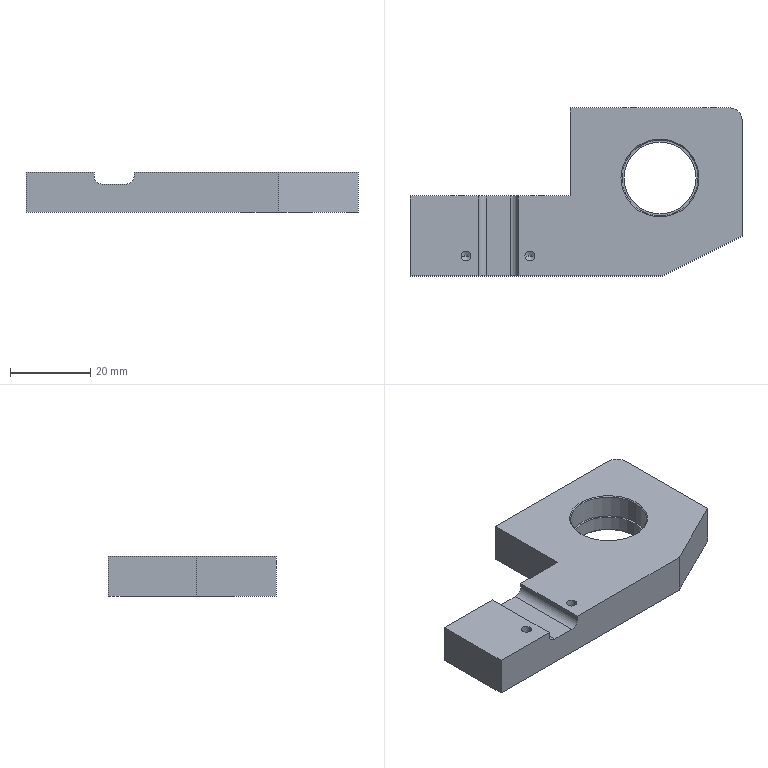Part | NX | features BREP 1 | 1 solid | 49 faces | box 83 x 42 x 10 mm | volume 21285 mm3 | cylinder 19 | cone 16 | plane 14 | commonest cylinder face diameters 3.3 x8 2.5 x4 4 x2 18 x2 19 x2 6 x1
STEP:
#1=CARTESIAN_POINT('',(15.,10.909,0.));
#2=VERTEX_POINT('',#1);
#3=CARTESIAN_POINT('',(15.,11.9,-1.65));
#4=VERTEX_POINT('',#3);
#5=CARTESIAN_POINT('',(15.,11.9,-1.65));
#6=DIRECTION('',(0.,0.515,-0.8572));
#7=VECTOR('',#6,1000.);
#8=LINE('',#5,#7);
#9=EDGE_CURVE('',#2,#4,#8,.T.);
#10=ORIENTED_EDGE('',*,*,#9,.F.);
#11=CARTESIAN_POINT('',(15.,11.9,1.65));
#12=VERTEX_POINT('',#11);
#13=CARTESIAN_POINT('',(15.,11.9,1.65));
#14=DIRECTION('',(0.,0.515,0.8572));
#15=VECTOR('',#14,1000.);
#16=LINE('',#13,#15);
#17=EDGE_CURVE('',#2,#12,#16,.T.);
#18=ORIENTED_EDGE('',*,*,#17,.T.);
#19=CARTESIAN_POINT('',(16.543,11.9,0.5854));
#20=VERTEX_POINT('',#19);
#21=CARTESIAN_POINT('',(15.,11.9,0.));
#22=DIRECTION('',(0.,1.,0.));
#23=DIRECTION('',(0.,0.,1.));
#24=AXIS2_PLACEMENT_3D('',#21,#22,#23);
#25=CIRCLE('',#24,1.65);
#26=EDGE_CURVE('',#12,#20,#25,.T.);
#27=ORIENTED_EDGE('',*,*,#26,.T.);
#28=CARTESIAN_POINT('',(16.543,11.9,-0.5854));
#29=VERTEX_POINT('',#28);
#30=CARTESIAN_POINT('',(16.543,11.9,-0.5854));
#31=CARTESIAN_POINT('',(16.39,11.777,-0.4108));
#32=CARTESIAN_POINT('',(16.149,11.565,0.002229));
#33=CARTESIAN_POINT('',(16.389,11.776,0.41));
#34=CARTESIAN_POINT('',(16.543,11.9,0.5854));
#35=B_SPLINE_CURVE_WITH_KNOTS('',3,(#30,#31,#32,#33,#34),.UNSPECIFIED.,.F.,.F.,(4,1,4),(0.,0.5,1.),.UNSPECIFIED.);
#36=EDGE_CURVE('',#29,#20,#35,.T.);
#37=ORIENTED_EDGE('',*,*,#36,.F.);
#38=CARTESIAN_POINT('',(15.,11.9,0.));
#39=DIRECTION('',(0.,1.,0.));
#40=DIRECTION('',(0.,0.,1.));
#41=AXIS2_PLACEMENT_3D('',#38,#39,#40);
#42=CIRCLE('',#41,1.65);
#43=EDGE_CURVE('',#29,#4,#42,.T.);
#44=ORIENTED_EDGE('',*,*,#43,.T.);
#45=EDGE_LOOP('',(#10,#18,#27,#37,#44));
#46=FACE_BOUND('',#45,.T.);
#47=CARTESIAN_POINT('',(15.,11.9,0.));
#48=DIRECTION('',(0.,1.,0.));
#49=DIRECTION('',(0.,0.,1.));
#50=AXIS2_PLACEMENT_3D('',#47,#48,#49);
#51=CONICAL_SURFACE('',#50,1.65,1.03);
#52=ADVANCED_FACE('',(#46),#51,.F.);
#53=CARTESIAN_POINT('',(15.,22.,-1.65));
#54=VERTEX_POINT('',#53);
#55=CARTESIAN_POINT('',(15.,22.,-1.65));
#56=DIRECTION('',(0.,1.,0.));
#57=VECTOR('',#56,1000.);
#58=LINE('',#55,#57);
#59=EDGE_CURVE('',#54,#4,#58,.F.);
#60=ORIENTED_EDGE('',*,*,#59,.T.);
#61=ORIENTED_EDGE('',*,*,#43,.F.);
#62=CARTESIAN_POINT('',(16.543,11.9,-0.5854));
#63=CARTESIAN_POINT('',(16.684,12.014,-0.2124));
#64=CARTESIAN_POINT('',(16.684,12.014,0.2124));
#65=CARTESIAN_POINT('',(16.543,11.9,0.5854));
#66=B_SPLINE_CURVE_WITH_KNOTS('',3,(#62,#63,#64,#65),.UNSPECIFIED.,.F.,.F.,(4,4),(0.,1.),.UNSPECIFIED.);
#67=EDGE_CURVE('',#20,#29,#66,.F.);
#68=ORIENTED_EDGE('',*,*,#67,.F.);
#69=ORIENTED_EDGE('',*,*,#26,.F.);
#70=CARTESIAN_POINT('',(15.,22.,1.65));
#71=VERTEX_POINT('',#70);
#72=CARTESIAN_POINT('',(15.,22.,1.65));
#73=DIRECTION('',(0.,1.,0.));
#74=VECTOR('',#73,1000.);
#75=LINE('',#72,#74);
#76=EDGE_CURVE('',#71,#12,#75,.F.);
#77=ORIENTED_EDGE('',*,*,#76,.F.);
#78=CARTESIAN_POINT('',(15.,22.,0.));
#79=DIRECTION('',(0.,1.,0.));
#80=DIRECTION('',(0.,0.,1.));
#81=AXIS2_PLACEMENT_3D('',#78,#79,#80);
#82=CIRCLE('',#81,1.65);
#83=EDGE_CURVE('',#71,#54,#82,.T.);
#84=ORIENTED_EDGE('',*,*,#83,.T.);
#85=EDGE_LOOP('',(#60,#61,#68,#69,#77,#84));
#86=FACE_BOUND('',#85,.T.);
#87=CARTESIAN_POINT('',(15.,22.,0.));
#88=DIRECTION('',(0.,1.,0.));
#89=DIRECTION('',(0.,0.,1.));
#90=AXIS2_PLACEMENT_3D('',#87,#88,#89);
#91=CYLINDRICAL_SURFACE('',#90,1.65);
#92=ADVANCED_FACE('',(#86),#91,.F.);
#93=CARTESIAN_POINT('',(-11.25,-15.,5.));
#94=VERTEX_POINT('',#93);
#95=CARTESIAN_POINT('',(-11.25,-15.,-2.5));
#96=VERTEX_POINT('',#95);
#97=CARTESIAN_POINT('',(-11.25,-15.,5.));
#98=DIRECTION('',(0.,0.,1.));
#99=VECTOR('',#98,1000.);
#100=LINE('',#97,#99);
#101=EDGE_CURVE('',#94,#96,#100,.F.);
#102=ORIENTED_EDGE('',*,*,#101,.T.);
#103=CARTESIAN_POINT('',(-8.75,-15.,-2.5));
#104=VERTEX_POINT('',#103);
#105=CARTESIAN_POINT('',(-10.,-15.,-2.5));
#106=DIRECTION('',(0.,0.,1.));
#107=DIRECTION('',(1.,0.,0.));
#108=AXIS2_PLACEMENT_3D('',#105,#106,#107);
#109=CIRCLE('',#108,1.25);
#110=EDGE_CURVE('',#104,#96,#109,.T.);
#111=ORIENTED_EDGE('',*,*,#110,.F.);
#112=CARTESIAN_POINT('',(-8.75,-15.,5.));
#113=VERTEX_POINT('',#112);
#114=CARTESIAN_POINT('',(-8.75,-15.,5.));
#115=DIRECTION('',(0.,0.,1.));
#116=VECTOR('',#115,1000.);
#117=LINE('',#114,#116);
#118=EDGE_CURVE('',#113,#104,#117,.F.);
#119=ORIENTED_EDGE('',*,*,#118,.F.);
#120=CARTESIAN_POINT('',(-10.,-15.,5.));
#121=DIRECTION('',(0.,0.,1.));
#122=DIRECTION('',(1.,0.,0.));
#123=AXIS2_PLACEMENT_3D('',#120,#121,#122);
#124=CIRCLE('',#123,1.25);
#125=EDGE_CURVE('',#113,#94,#124,.T.);
#126=ORIENTED_EDGE('',*,*,#125,.T.);
#127=EDGE_LOOP('',(#102,#111,#119,#126));
#128=FACE_BOUND('',#127,.T.);
#129=CARTESIAN_POINT('',(-10.,-15.,5.));
#130=DIRECTION('',(0.,0.,1.));
#131=DIRECTION('',(1.,0.,0.));
#132=AXIS2_PLACEMENT_3D('',#129,#130,#131);
#133=CYLINDRICAL_SURFACE('',#132,1.25);
#134=ADVANCED_FACE('',(#128),#133,.F.);
#135=CARTESIAN_POINT('',(-10.,-15.,-3.251));
#136=VERTEX_POINT('',#135);
#137=CARTESIAN_POINT('',(-11.25,-15.,-2.5));
#138=DIRECTION('',(-0.8572,0.,0.515));
#139=VECTOR('',#138,1000.);
#140=LINE('',#137,#139);
#141=EDGE_CURVE('',#136,#96,#140,.T.);
#142=ORIENTED_EDGE('',*,*,#141,.F.);
#143=CARTESIAN_POINT('',(-8.75,-15.,-2.5));
#144=DIRECTION('',(0.8572,0.,0.515));
#145=VECTOR('',#144,1000.);
#146=LINE('',#143,#145);
#147=EDGE_CURVE('',#136,#104,#146,.T.);
#148=ORIENTED_EDGE('',*,*,#147,.T.);
#149=ORIENTED_EDGE('',*,*,#110,.T.);
#150=EDGE_LOOP('',(#142,#148,#149));
#151=FACE_BOUND('',#150,.T.);
#152=CARTESIAN_POINT('',(-10.,-15.,-2.5));
#153=DIRECTION('',(0.,0.,1.));
#154=DIRECTION('',(1.,0.,0.));
#155=AXIS2_PLACEMENT_3D('',#152,#153,#154);
#156=CONICAL_SURFACE('',#155,1.25,1.03);
#157=ADVANCED_FACE('',(#151),#156,.F.);
#158=CARTESIAN_POINT('',(-27.25,-15.,5.));
#159=VERTEX_POINT('',#158);
#160=CARTESIAN_POINT('',(-27.25,-15.,-2.5));
#161=VERTEX_POINT('',#160);
#162=CARTESIAN_POINT('',(-27.25,-15.,5.));
#163=DIRECTION('',(0.,0.,1.));
#164=VECTOR('',#163,1000.);
#165=LINE('',#162,#164);
#166=EDGE_CURVE('',#159,#161,#165,.F.);
#167=ORIENTED_EDGE('',*,*,#166,.T.);
#168=CARTESIAN_POINT('',(-24.75,-15.,-2.5));
#169=VERTEX_POINT('',#168);
#170=CARTESIAN_POINT('',(-26.,-15.,-2.5));
#171=DIRECTION('',(0.,0.,1.));
#172=DIRECTION('',(1.,0.,0.));
#173=AXIS2_PLACEMENT_3D('',#170,#171,#172);
#174=CIRCLE('',#173,1.25);
#175=EDGE_CURVE('',#169,#161,#174,.T.);
#176=ORIENTED_EDGE('',*,*,#175,.F.);
#177=CARTESIAN_POINT('',(-24.75,-15.,5.));
#178=VERTEX_POINT('',#177);
#179=CARTESIAN_POINT('',(-24.75,-15.,5.));
#180=DIRECTION('',(0.,0.,1.));
#181=VECTOR('',#180,1000.);
#182=LINE('',#179,#181);
#183=EDGE_CURVE('',#178,#169,#182,.F.);
#184=ORIENTED_EDGE('',*,*,#183,.F.);
#185=CARTESIAN_POINT('',(-26.,-15.,5.));
#186=DIRECTION('',(0.,0.,1.));
#187=DIRECTION('',(1.,0.,0.));
#188=AXIS2_PLACEMENT_3D('',#185,#186,#187);
#189=CIRCLE('',#188,1.25);
#190=EDGE_CURVE('',#178,#159,#189,.T.);
#191=ORIENTED_EDGE('',*,*,#190,.T.);
#192=EDGE_LOOP('',(#167,#176,#184,#191));
#193=FACE_BOUND('',#192,.T.);
#194=CARTESIAN_POINT('',(-26.,-15.,5.));
#195=DIRECTION('',(0.,0.,1.));
#196=DIRECTION('',(1.,0.,0.));
#197=AXIS2_PLACEMENT_3D('',#194,#195,#196);
#198=CYLINDRICAL_SURFACE('',#197,1.25);
#199=ADVANCED_FACE('',(#193),#198,.F.);
#200=CARTESIAN_POINT('',(-26.,-15.,-3.251));
#201=VERTEX_POINT('',#200);
#202=CARTESIAN_POINT('',(-27.25,-15.,-2.5));
#203=DIRECTION('',(-0.8572,0.,0.515));
#204=VECTOR('',#203,1000.);
#205=LINE('',#202,#204);
#206=EDGE_CURVE('',#201,#161,#205,.T.);
#207=ORIENTED_EDGE('',*,*,#206,.F.);
#208=CARTESIAN_POINT('',(-24.75,-15.,-2.5));
#209=DIRECTION('',(0.8572,0.,0.515));
#210=VECTOR('',#209,1000.);
#211=LINE('',#208,#210);
#212=EDGE_CURVE('',#201,#169,#211,.T.);
#213=ORIENTED_EDGE('',*,*,#212,.T.);
#214=ORIENTED_EDGE('',*,*,#175,.T.);
#215=EDGE_LOOP('',(#207,#213,#214));
#216=FACE_BOUND('',#215,.T.);
#217=CARTESIAN_POINT('',(-26.,-15.,-2.5));
#218=DIRECTION('',(0.,0.,1.));
#219=DIRECTION('',(1.,0.,0.));
#220=AXIS2_PLACEMENT_3D('',#217,#218,#219);
#221=CONICAL_SURFACE('',#220,1.25,1.03);
#222=ADVANCED_FACE('',(#216),#221,.F.);
#223=CARTESIAN_POINT('',(-23.,0.,5.));
#224=VERTEX_POINT('',#223);
#225=CARTESIAN_POINT('',(-23.,-20.,5.));
#226=VERTEX_POINT('',#225);
#227=CARTESIAN_POINT('',(-23.,0.,5.));
#228=DIRECTION('',(0.,-1.,0.));
#229=VECTOR('',#228,1000.);
#230=LINE('',#227,#229);
#231=EDGE_CURVE('',#224,#226,#230,.T.);
#232=ORIENTED_EDGE('',*,*,#231,.T.);
#233=CARTESIAN_POINT('',(-23.,-20.,4.));
#234=VERTEX_POINT('',#233);
#235=CARTESIAN_POINT('',(-23.,-20.,8.));
#236=DIRECTION('',(0.,0.,-1.));
#237=VECTOR('',#236,1000.);
#238=LINE('',#235,#237);
#239=EDGE_CURVE('',#226,#234,#238,.T.);
#240=ORIENTED_EDGE('',*,*,#239,.T.);
#241=CARTESIAN_POINT('',(-23.,0.,4.));
#242=VERTEX_POINT('',#241);
#243=CARTESIAN_POINT('',(-23.,22.,4.));
#244=DIRECTION('',(0.,-1.,0.));
#245=VECTOR('',#244,1000.);
#246=LINE('',#243,#245);
#247=EDGE_CURVE('',#242,#234,#246,.T.);
#248=ORIENTED_EDGE('',*,*,#247,.F.);
#249=CARTESIAN_POINT('',(-23.,0.,5.));
#250=DIRECTION('',(0.,0.,-1.));
#251=VECTOR('',#250,1000.);
#252=LINE('',#249,#251);
#253=EDGE_CURVE('',#224,#242,#252,.T.);
#254=ORIENTED_EDGE('',*,*,#253,.F.);
#255=EDGE_LOOP('',(#232,#240,#248,#254));
#256=FACE_BOUND('',#255,.T.);
#257=CARTESIAN_POINT('',(-23.,22.,8.));
#258=DIRECTION('',(-1.,0.,0.));
#259=DIRECTION('',(0.,-1.,0.));
#260=AXIS2_PLACEMENT_3D('',#257,#258,#259);
#261=PLANE('',#260);
#262=ADVANCED_FACE('',(#256),#261,.F.);
#263=CARTESIAN_POINT('',(-13.,0.,4.));
#264=VERTEX_POINT('',#263);
#265=CARTESIAN_POINT('',(-13.,-20.,4.));
#266=VERTEX_POINT('',#265);
#267=CARTESIAN_POINT('',(-13.,22.,4.));
#268=DIRECTION('',(0.,-1.,0.));
#269=VECTOR('',#268,1000.);
#270=LINE('',#267,#269);
#271=EDGE_CURVE('',#264,#266,#270,.T.);
#272=ORIENTED_EDGE('',*,*,#271,.T.);
#273=CARTESIAN_POINT('',(-13.,-20.,5.));
#274=VERTEX_POINT('',#273);
#275=CARTESIAN_POINT('',(-13.,-20.,8.));
#276=DIRECTION('',(0.,0.,1.));
#277=VECTOR('',#276,1000.);
#278=LINE('',#275,#277);
#279=EDGE_CURVE('',#266,#274,#278,.T.);
#280=ORIENTED_EDGE('',*,*,#279,.T.);
#281=CARTESIAN_POINT('',(-13.,0.,5.));
#282=VERTEX_POINT('',#281);
#283=CARTESIAN_POINT('',(-13.,0.,5.));
#284=DIRECTION('',(0.,1.,0.));
#285=VECTOR('',#284,1000.);
#286=LINE('',#283,#285);
#287=EDGE_CURVE('',#274,#282,#286,.T.);
#288=ORIENTED_EDGE('',*,*,#287,.T.);
#289=CARTESIAN_POINT('',(-13.,0.,5.));
#290=DIRECTION('',(0.,0.,1.));
#291=VECTOR('',#290,1000.);
#292=LINE('',#289,#291);
#293=EDGE_CURVE('',#264,#282,#292,.T.);
#294=ORIENTED_EDGE('',*,*,#293,.F.);
#295=EDGE_LOOP('',(#272,#280,#288,#294));
#296=FACE_BOUND('',#295,.T.);
#297=CARTESIAN_POINT('',(-13.,22.,8.));
#298=DIRECTION('',(1.,0.,0.));
#299=DIRECTION('',(0.,1.,0.));
#300=AXIS2_PLACEMENT_3D('',#297,#298,#299);
#301=PLANE('',#300);
#302=ADVANCED_FACE('',(#296),#301,.F.);
#303=ORIENTED_EDGE('',*,*,#247,.T.);
#304=CARTESIAN_POINT('',(-21.,-20.,2.));
#305=VERTEX_POINT('',#304);
#306=CARTESIAN_POINT('',(-21.,-20.,4.));
#307=DIRECTION('',(0.,-1.,0.));
#308=DIRECTION('',(1.,0.,0.));
#309=AXIS2_PLACEMENT_3D('',#306,#307,#308);
#310=CIRCLE('',#309,2.);
#311=EDGE_CURVE('',#234,#305,#310,.T.);
#312=ORIENTED_EDGE('',*,*,#311,.T.);
#313=CARTESIAN_POINT('',(-21.,0.,2.));
#314=VERTEX_POINT('',#313);
#315=CARTESIAN_POINT('',(-21.,22.,2.));
#316=DIRECTION('',(0.,-1.,0.));
#317=VECTOR('',#316,1000.);
#318=LINE('',#315,#317);
#319=EDGE_CURVE('',#314,#305,#318,.T.);
#320=ORIENTED_EDGE('',*,*,#319,.F.);
#321=CARTESIAN_POINT('',(-21.,0.,4.));
#322=DIRECTION('',(0.,-1.,0.));
#323=DIRECTION('',(0.,0.,-1.));
#324=AXIS2_PLACEMENT_3D('',#321,#322,#323);
#325=CIRCLE('',#324,2.);
#326=EDGE_CURVE('',#242,#314,#325,.T.);
#327=ORIENTED_EDGE('',*,*,#326,.F.);
#328=EDGE_LOOP('',(#303,#312,#320,#327));
#329=FACE_BOUND('',#328,.T.);
#330=CARTESIAN_POINT('',(-21.,22.,4.));
#331=DIRECTION('',(0.,-1.,0.));
#332=DIRECTION('',(1.,0.,0.));
#333=AXIS2_PLACEMENT_3D('',#330,#331,#332);
#334=CYLINDRICAL_SURFACE('',#333,2.);
#335=ADVANCED_FACE('',(#329),#334,.F.);
#336=ORIENTED_EDGE('',*,*,#319,.T.);
#337=CARTESIAN_POINT('',(-15.,-20.,2.));
#338=VERTEX_POINT('',#337);
#339=CARTESIAN_POINT('',(-15.,-20.,2.));
#340=DIRECTION('',(1.,0.,0.));
#341=VECTOR('',#340,1000.);
#342=LINE('',#339,#341);
#343=EDGE_CURVE('',#305,#338,#342,.T.);
#344=ORIENTED_EDGE('',*,*,#343,.T.);
#345=CARTESIAN_POINT('',(-15.,0.,2.));
#346=VERTEX_POINT('',#345);
#347=CARTESIAN_POINT('',(-15.,22.,2.));
#348=DIRECTION('',(0.,-1.,0.));
#349=VECTOR('',#348,1000.);
#350=LINE('',#347,#349);
#351=EDGE_CURVE('',#346,#338,#350,.T.);
#352=ORIENTED_EDGE('',*,*,#351,.F.);
#353=CARTESIAN_POINT('',(-40.,0.,2.));
#354=DIRECTION('',(1.,0.,0.));
#355=VECTOR('',#354,1000.);
#356=LINE('',#353,#355);
#357=EDGE_CURVE('',#314,#346,#356,.T.);
#358=ORIENTED_EDGE('',*,*,#357,.F.);
#359=EDGE_LOOP('',(#336,#344,#352,#358));
#360=FACE_BOUND('',#359,.T.);
#361=CARTESIAN_POINT('',(-15.,22.,2.));
#362=DIRECTION('',(0.,0.,-1.));
#363=DIRECTION('',(-1.,0.,0.));
#364=AXIS2_PLACEMENT_3D('',#361,#362,#363);
#365=PLANE('',#364);
#366=ADVANCED_FACE('',(#360),#365,.F.);
#367=ORIENTED_EDGE('',*,*,#351,.T.);
#368=CARTESIAN_POINT('',(-15.,-20.,4.));
#369=DIRECTION('',(0.,-1.,0.));
#370=DIRECTION('',(1.,0.,0.));
#371=AXIS2_PLACEMENT_3D('',#368,#369,#370);
#372=CIRCLE('',#371,2.);
#373=EDGE_CURVE('',#338,#266,#372,.T.);
#374=ORIENTED_EDGE('',*,*,#373,.T.);
#375=ORIENTED_EDGE('',*,*,#271,.F.);
#376=CARTESIAN_POINT('',(-15.,0.,4.));
#377=DIRECTION('',(0.,-1.,0.));
#378=DIRECTION('',(0.,0.,-1.));
#379=AXIS2_PLACEMENT_3D('',#376,#377,#378);
#380=CIRCLE('',#379,2.);
#381=EDGE_CURVE('',#346,#264,#380,.T.);
#382=ORIENTED_EDGE('',*,*,#381,.F.);
#383=EDGE_LOOP('',(#367,#374,#375,#382));
#384=FACE_BOUND('',#383,.T.);
#385=CARTESIAN_POINT('',(-15.,22.,4.));
#386=DIRECTION('',(0.,-1.,0.));
#387=DIRECTION('',(1.,0.,0.));
#388=AXIS2_PLACEMENT_3D('',#385,#386,#387);
#389=CYLINDRICAL_SURFACE('',#388,2.);
#390=ADVANCED_FACE('',(#384),#389,.F.);
#391=CARTESIAN_POINT('',(12.75,4.5,5.));
#392=VERTEX_POINT('',#391);
#393=CARTESIAN_POINT('',(13.,4.5,4.75));
#394=VERTEX_POINT('',#393);
#395=CARTESIAN_POINT('',(13.,4.5,4.75));
#396=DIRECTION('',(-0.7071,0.,0.7071));
#397=VECTOR('',#396,1000.);
#398=LINE('',#395,#397);
#399=EDGE_CURVE('',#392,#394,#398,.F.);
#400=ORIENTED_EDGE('',*,*,#399,.T.);
#401=CARTESIAN_POINT('',(32.,4.5,4.75));
#402=VERTEX_POINT('',#401);
#403=CARTESIAN_POINT('',(22.5,4.5,4.75));
#404=DIRECTION('',(0.,0.,1.));
#405=DIRECTION('',(1.,0.,0.));
#406=AXIS2_PLACEMENT_3D('',#403,#404,#405);
#407=CIRCLE('',#406,9.5);
#408=EDGE_CURVE('',#402,#394,#407,.T.);
#409=ORIENTED_EDGE('',*,*,#408,.F.);
#410=CARTESIAN_POINT('',(32.25,4.5,5.));
#411=VERTEX_POINT('',#410);
#412=CARTESIAN_POINT('',(32.,4.5,4.75));
#413=DIRECTION('',(0.7071,0.,0.7071));
#414=VECTOR('',#413,1000.);
#415=LINE('',#412,#414);
#416=EDGE_CURVE('',#411,#402,#415,.F.);
#417=ORIENTED_EDGE('',*,*,#416,.F.);
#418=CARTESIAN_POINT('',(22.5,4.5,5.));
#419=DIRECTION('',(0.,0.,-1.));
#420=DIRECTION('',(1.,0.,0.));
#421=AXIS2_PLACEMENT_3D('',#418,#419,#420);
#422=CIRCLE('',#421,9.75);
#423=EDGE_CURVE('',#392,#411,#422,.T.);
#424=ORIENTED_EDGE('',*,*,#423,.F.);
#425=EDGE_LOOP('',(#400,#409,#417,#424));
#426=FACE_BOUND('',#425,.T.);
#427=CARTESIAN_POINT('',(22.5,4.5,4.75));
#428=DIRECTION('',(0.,0.,1.));
#429=DIRECTION('',(1.,0.,0.));
#430=AXIS2_PLACEMENT_3D('',#427,#428,#429);
#431=CONICAL_SURFACE('',#430,9.5,0.7854);
#432=ADVANCED_FACE('',(#426),#431,.F.);
#433=CARTESIAN_POINT('',(31.5,4.5,-4.75));
#434=VERTEX_POINT('',#433);
#435=CARTESIAN_POINT('',(31.75,4.5,-5.));
#436=VERTEX_POINT('',#435);
#437=CARTESIAN_POINT('',(31.75,4.5,-5.));
#438=DIRECTION('',(0.7071,0.,-0.7071));
#439=VECTOR('',#438,1000.);
#440=LINE('',#437,#439);
#441=EDGE_CURVE('',#434,#436,#440,.T.);
#442=ORIENTED_EDGE('',*,*,#441,.F.);
#443=CARTESIAN_POINT('',(13.5,4.5,-4.75));
#444=VERTEX_POINT('',#443);
#445=CARTESIAN_POINT('',(22.5,4.5,-4.75));
#446=DIRECTION('',(0.,0.,-1.));
#447=DIRECTION('',(1.,0.,0.));
#448=AXIS2_PLACEMENT_3D('',#445,#446,#447);
#449=CIRCLE('',#448,9.);
#450=EDGE_CURVE('',#444,#434,#449,.T.);
#451=ORIENTED_EDGE('',*,*,#450,.F.);
#452=CARTESIAN_POINT('',(13.25,4.5,-5.));
#453=VERTEX_POINT('',#452);
#454=CARTESIAN_POINT('',(13.25,4.5,-5.));
#455=DIRECTION('',(-0.7071,0.,-0.7071));
#456=VECTOR('',#455,1000.);
#457=LINE('',#454,#456);
#458=EDGE_CURVE('',#444,#453,#457,.T.);
#459=ORIENTED_EDGE('',*,*,#458,.T.);
#460=CARTESIAN_POINT('',(22.5,4.5,-5.));
#461=DIRECTION('',(0.,0.,1.));
#462=DIRECTION('',(1.,0.,0.));
#463=AXIS2_PLACEMENT_3D('',#460,#461,#462);
#464=CIRCLE('',#463,9.25);
#465=EDGE_CURVE('',#436,#453,#464,.T.);
#466=ORIENTED_EDGE('',*,*,#465,.F.);
#467=EDGE_LOOP('',(#442,#451,#459,#466));
#468=FACE_BOUND('',#467,.T.);
#469=CARTESIAN_POINT('',(22.5,4.5,-5.));
#470=DIRECTION('',(0.,0.,-1.));
#471=DIRECTION('',(-1.,0.,0.));
#472=AXIS2_PLACEMENT_3D('',#469,#470,#471);
#473=CONICAL_SURFACE('',#472,9.25,0.7854);
#474=ADVANCED_FACE('',(#468),#473,.F.);
#475=CARTESIAN_POINT('',(35.,22.,-1.65));
#476=VERTEX_POINT('',#475);
#477=CARTESIAN_POINT('',(35.,11.9,-1.65));
#478=VERTEX_POINT('',#477);
#479=CARTESIAN_POINT('',(35.,22.,-1.65));
#480=DIRECTION('',(0.,1.,0.));
#481=VECTOR('',#480,1000.);
#482=LINE('',#479,#481);
#483=EDGE_CURVE('',#476,#478,#482,.F.);
#484=ORIENTED_EDGE('',*,*,#483,.T.);
#485=CARTESIAN_POINT('',(35.,11.9,1.65));
#486=VERTEX_POINT('',#485);
#487=CARTESIAN_POINT('',(35.,11.9,0.));
#488=DIRECTION('',(0.,1.,0.));
#489=DIRECTION('',(0.,0.,1.));
#490=AXIS2_PLACEMENT_3D('',#487,#488,#489);
#491=CIRCLE('',#490,1.65);
#492=EDGE_CURVE('',#486,#478,#491,.T.);
#493=ORIENTED_EDGE('',*,*,#492,.F.);
#494=CARTESIAN_POINT('',(35.,22.,1.65));
#495=VERTEX_POINT('',#494);
#496=CARTESIAN_POINT('',(35.,22.,1.65));
#497=DIRECTION('',(0.,1.,0.));
#498=VECTOR('',#497,1000.);
#499=LINE('',#496,#498);
#500=EDGE_CURVE('',#495,#486,#499,.F.);
#501=ORIENTED_EDGE('',*,*,#500,.F.);
#502=CARTESIAN_POINT('',(35.,22.,0.));
#503=DIRECTION('',(0.,1.,0.));
#504=DIRECTION('',(0.,0.,1.));
#505=AXIS2_PLACEMENT_3D('',#502,#503,#504);
#506=CIRCLE('',#505,1.65);
#507=EDGE_CURVE('',#495,#476,#506,.T.);
#508=ORIENTED_EDGE('',*,*,#507,.T.);
#509=EDGE_LOOP('',(#484,#493,#501,#508));
#510=FACE_BOUND('',#509,.T.);
#511=CARTESIAN_POINT('',(35.,22.,0.));
#512=DIRECTION('',(0.,1.,0.));
#513=DIRECTION('',(0.,0.,1.));
#514=AXIS2_PLACEMENT_3D('',#511,#512,#513);
#515=CYLINDRICAL_SURFACE('',#514,1.65);
#516=ADVANCED_FACE('',(#510),#515,.F.);
#517=CARTESIAN_POINT('',(35.,10.909,0.));
#518=VERTEX_POINT('',#517);
#519=CARTESIAN_POINT('',(35.,11.9,-1.65));
#520=DIRECTION('',(0.,0.515,-0.8572));
#521=VECTOR('',#520,1000.);
#522=LINE('',#519,#521);
#523=EDGE_CURVE('',#518,#478,#522,.T.);
#524=ORIENTED_EDGE('',*,*,#523,.F.);
#525=CARTESIAN_POINT('',(35.,11.9,1.65));
#526=DIRECTION('',(0.,0.515,0.8572));
#527=VECTOR('',#526,1000.);
#528=LINE('',#525,#527);
#529=EDGE_CURVE('',#518,#486,#528,.T.);
#530=ORIENTED_EDGE('',*,*,#529,.T.);
#531=ORIENTED_EDGE('',*,*,#492,.T.);
#532=EDGE_LOOP('',(#524,#530,#531));
#533=FACE_BOUND('',#532,.T.);
#534=CARTESIAN_POINT('',(35.,11.9,0.));
#535=DIRECTION('',(0.,1.,0.));
#536=DIRECTION('',(0.,0.,1.));
#537=AXIS2_PLACEMENT_3D('',#534,#535,#536);
#538=CONICAL_SURFACE('',#537,1.65,1.03);
#539=ADVANCED_FACE('',(#533),#538,.F.);
#540=CARTESIAN_POINT('',(43.,19.,5.));
#541=VERTEX_POINT('',#540);
#542=CARTESIAN_POINT('',(40.,22.,5.));
#543=VERTEX_POINT('',#542);
#544=CARTESIAN_POINT('',(40.,19.,5.));
#545=DIRECTION('',(0.,0.,1.));
#546=DIRECTION('',(1.,0.,0.));
#547=AXIS2_PLACEMENT_3D('',#544,#545,#546);
#548=CIRCLE('',#547,3.);
#549=EDGE_CURVE('',#541,#543,#548,.T.);
#550=ORIENTED_EDGE('',*,*,#549,.F.);
#551=CARTESIAN_POINT('',(43.,19.,-5.));
#552=VERTEX_POINT('',#551);
#553=CARTESIAN_POINT('',(43.,19.,5.));
#554=DIRECTION('',(0.,0.,1.));
#555=VECTOR('',#554,1000.);
#556=LINE('',#553,#555);
#557=EDGE_CURVE('',#552,#541,#556,.T.);
#558=ORIENTED_EDGE('',*,*,#557,.F.);
#559=CARTESIAN_POINT('',(40.,22.,-5.));
#560=VERTEX_POINT('',#559);
#561=CARTESIAN_POINT('',(40.,19.,-5.));
#562=DIRECTION('',(0.,0.,-1.));
#563=DIRECTION('',(1.,0.,0.));
#564=AXIS2_PLACEMENT_3D('',#561,#562,#563);
#565=CIRCLE('',#564,3.);
#566=EDGE_CURVE('',#560,#552,#565,.T.);
#567=ORIENTED_EDGE('',*,*,#566,.F.);
#568=CARTESIAN_POINT('',(40.,22.,5.));
#569=DIRECTION('',(0.,0.,-1.));
#570=VECTOR('',#569,1000.);
#571=LINE('',#568,#570);
#572=EDGE_CURVE('',#543,#560,#571,.T.);
#573=ORIENTED_EDGE('',*,*,#572,.F.);
#574=EDGE_LOOP('',(#550,#558,#567,#573));
#575=FACE_BOUND('',#574,.T.);
#576=CARTESIAN_POINT('',(40.,19.,5.));
#577=DIRECTION('',(0.,0.,-1.));
#578=DIRECTION('',(-1.,0.,0.));
#579=AXIS2_PLACEMENT_3D('',#576,#577,#578);
#580=CYLINDRICAL_SURFACE('',#579,3.);
#581=ADVANCED_FACE('',(#575),#580,.T.);
#582=CARTESIAN_POINT('',(13.5,4.5,-1.));
#583=VERTEX_POINT('',#582);
#584=CARTESIAN_POINT('',(13.5,4.5,-5.));
#585=DIRECTION('',(0.,0.,1.));
#586=VECTOR('',#585,1000.);
#587=LINE('',#584,#586);
#588=EDGE_CURVE('',#583,#444,#587,.F.);
#589=ORIENTED_EDGE('',*,*,#588,.T.);
#590=ORIENTED_EDGE('',*,*,#450,.T.);
#591=CARTESIAN_POINT('',(31.5,4.5,-1.));
#592=VERTEX_POINT('',#591);
#593=CARTESIAN_POINT('',(31.5,4.5,-5.));
#594=DIRECTION('',(0.,0.,1.));
#595=VECTOR('',#594,1000.);
#596=LINE('',#593,#595);
#597=EDGE_CURVE('',#592,#434,#596,.F.);
#598=ORIENTED_EDGE('',*,*,#597,.F.);
#599=CARTESIAN_POINT('',(22.5,4.5,-1.));
#600=DIRECTION('',(0.,0.,1.));
#601=DIRECTION('',(1.,0.,0.));
#602=AXIS2_PLACEMENT_3D('',#599,#600,#601);
#603=CIRCLE('',#602,9.);
#604=EDGE_CURVE('',#592,#583,#603,.T.);
#605=ORIENTED_EDGE('',*,*,#604,.T.);
#606=EDGE_LOOP('',(#589,#590,#598,#605));
#607=FACE_BOUND('',#606,.T.);
#608=CARTESIAN_POINT('',(22.5,4.5,-5.));
#609=DIRECTION('',(0.,0.,1.));
#610=DIRECTION('',(1.,0.,0.));
#611=AXIS2_PLACEMENT_3D('',#608,#609,#610);
#612=CYLINDRICAL_SURFACE('',#611,9.);
#613=ADVANCED_FACE('',(#607),#612,.F.);
#614=CARTESIAN_POINT('',(32.,4.5,-1.));
#615=VERTEX_POINT('',#614);
#616=CARTESIAN_POINT('',(13.,4.5,-1.));
#617=VERTEX_POINT('',#616);
#618=CARTESIAN_POINT('',(22.5,4.5,-1.));
#619=DIRECTION('',(0.,0.,1.));
#620=DIRECTION('',(1.,0.,0.));
#621=AXIS2_PLACEMENT_3D('',#618,#619,#620);
#622=CIRCLE('',#621,9.5);
#623=EDGE_CURVE('',#615,#617,#622,.T.);
#624=ORIENTED_EDGE('',*,*,#623,.T.);
#625=CARTESIAN_POINT('',(22.5,4.5,-1.));
#626=DIRECTION('',(0.,0.,1.));
#627=DIRECTION('',(1.,0.,0.));
#628=AXIS2_PLACEMENT_3D('',#625,#626,#627);
#629=CIRCLE('',#628,9.5);
#630=EDGE_CURVE('',#617,#615,#629,.T.);
#631=ORIENTED_EDGE('',*,*,#630,.T.);
#632=EDGE_LOOP('',(#624,#631));
#633=FACE_BOUND('',#632,.T.);
#634=ORIENTED_EDGE('',*,*,#604,.F.);
#635=CARTESIAN_POINT('',(22.5,4.5,-1.));
#636=DIRECTION('',(0.,0.,1.));
#637=DIRECTION('',(1.,0.,0.));
#638=AXIS2_PLACEMENT_3D('',#635,#636,#637);
#639=CIRCLE('',#638,9.);
#640=EDGE_CURVE('',#583,#592,#639,.T.);
#641=ORIENTED_EDGE('',*,*,#640,.F.);
#642=EDGE_LOOP('',(#634,#641));
#643=FACE_BOUND('',#642,.T.);
#644=CARTESIAN_POINT('',(0.,0.,-1.));
#645=DIRECTION('',(0.,0.,1.));
#646=DIRECTION('',(1.,0.,0.));
#647=AXIS2_PLACEMENT_3D('',#644,#645,#646);
#648=PLANE('',#647);
#649=ADVANCED_FACE('',(#633,#643),#648,.T.);
#650=ORIENTED_EDGE('',*,*,#36,.T.);
#651=ORIENTED_EDGE('',*,*,#67,.T.);
#652=EDGE_LOOP('',(#650,#651));
#653=FACE_BOUND('',#652,.T.);
#654=CARTESIAN_POINT('',(13.,4.5,-1.));
#655=DIRECTION('',(0.,0.,1.));
#656=VECTOR('',#655,1000.);
#657=LINE('',#654,#656);
#658=EDGE_CURVE('',#394,#617,#657,.F.);
#659=ORIENTED_EDGE('',*,*,#658,.T.);
#660=ORIENTED_EDGE('',*,*,#623,.F.);
#661=CARTESIAN_POINT('',(32.,4.5,-1.));
#662=DIRECTION('',(0.,0.,1.));
#663=VECTOR('',#662,1000.);
#664=LINE('',#661,#663);
#665=EDGE_CURVE('',#402,#615,#664,.F.);
#666=ORIENTED_EDGE('',*,*,#665,.F.);
#667=ORIENTED_EDGE('',*,*,#408,.T.);
#668=EDGE_LOOP('',(#659,#660,#666,#667));
#669=FACE_BOUND('',#668,.T.);
#670=CARTESIAN_POINT('',(22.5,4.5,-1.));
#671=DIRECTION('',(0.,0.,1.));
#672=DIRECTION('',(1.,0.,0.));
#673=AXIS2_PLACEMENT_3D('',#670,#671,#672);
#674=CYLINDRICAL_SURFACE('',#673,9.5);
#675=ADVANCED_FACE('',(#653,#669),#674,.F.);
#676=CARTESIAN_POINT('',(23.,-20.,5.));
#677=VERTEX_POINT('',#676);
#678=CARTESIAN_POINT('',(43.,-10.,5.));
#679=VERTEX_POINT('',#678);
#680=CARTESIAN_POINT('',(12.6,-25.2,5.));
#681=DIRECTION('',(0.8944,0.4472,0.));
#682=VECTOR('',#681,1000.);
#683=LINE('',#680,#682);
#684=EDGE_CURVE('',#677,#679,#683,.T.);
#685=ORIENTED_EDGE('',*,*,#684,.F.);
#686=CARTESIAN_POINT('',(23.,-20.,-5.));
#687=VERTEX_POINT('',#686);
#688=CARTESIAN_POINT('',(23.,-20.,5.));
#689=DIRECTION('',(0.,0.,1.));
#690=VECTOR('',#689,1000.);
#691=LINE('',#688,#690);
#692=EDGE_CURVE('',#687,#677,#691,.T.);
#693=ORIENTED_EDGE('',*,*,#692,.F.);
#694=CARTESIAN_POINT('',(43.,-10.,-5.));
#695=VERTEX_POINT('',#694);
#696=CARTESIAN_POINT('',(43.,-10.,-5.));
#697=DIRECTION('',(-0.8944,-0.4472,0.));
#698=VECTOR('',#697,1000.);
#699=LINE('',#696,#698);
#700=EDGE_CURVE('',#695,#687,#699,.T.);
#701=ORIENTED_EDGE('',*,*,#700,.F.);
#702=CARTESIAN_POINT('',(43.,-10.,5.));
#703=DIRECTION('',(0.,0.,-1.));
#704=VECTOR('',#703,1000.);
#705=LINE('',#702,#704);
#706=EDGE_CURVE('',#679,#695,#705,.T.);
#707=ORIENTED_EDGE('',*,*,#706,.F.);
#708=EDGE_LOOP('',(#685,#693,#701,#707));
#709=FACE_BOUND('',#708,.T.);
#710=CARTESIAN_POINT('',(43.,-10.,5.));
#711=DIRECTION('',(-0.4472,0.8944,0.));
#712=DIRECTION('',(0.,0.,-1.));
#713=AXIS2_PLACEMENT_3D('',#710,#711,#712);
#714=PLANE('',#713);
#715=ADVANCED_FACE('',(#709),#714,.F.);
#716=CARTESIAN_POINT('',(-8.,0.,-1.65));
#717=VERTEX_POINT('',#716);
#718=CARTESIAN_POINT('',(-8.,-12.1,-1.65));
#719=VERTEX_POINT('',#718);
#720=CARTESIAN_POINT('',(-8.,0.,-1.65));
#721=DIRECTION('',(0.,1.,0.));
#722=VECTOR('',#721,1000.);
#723=LINE('',#720,#722);
#724=EDGE_CURVE('',#717,#719,#723,.F.);
#725=ORIENTED_EDGE('',*,*,#724,.T.);
#726=CARTESIAN_POINT('',(-8.,-12.1,1.65));
#727=VERTEX_POINT('',#726);
#728=CARTESIAN_POINT('',(-8.,-12.1,0.));
#729=DIRECTION('',(0.,1.,0.));
#730=DIRECTION('',(0.,0.,1.));
#731=AXIS2_PLACEMENT_3D('',#728,#729,#730);
#732=CIRCLE('',#731,1.65);
#733=EDGE_CURVE('',#727,#719,#732,.T.);
#734=ORIENTED_EDGE('',*,*,#733,.F.);
#735=CARTESIAN_POINT('',(-8.,0.,1.65));
#736=VERTEX_POINT('',#735);
#737=CARTESIAN_POINT('',(-8.,0.,1.65));
#738=DIRECTION('',(0.,1.,0.));
#739=VECTOR('',#738,1000.);
#740=LINE('',#737,#739);
#741=EDGE_CURVE('',#736,#727,#740,.F.);
#742=ORIENTED_EDGE('',*,*,#741,.F.);
#743=CARTESIAN_POINT('',(-8.,0.,0.));
#744=DIRECTION('',(0.,1.,0.));
#745=DIRECTION('',(0.,0.,1.));
#746=AXIS2_PLACEMENT_3D('',#743,#744,#745);
#747=CIRCLE('',#746,1.65);
#748=EDGE_CURVE('',#736,#717,#747,.T.);
#749=ORIENTED_EDGE('',*,*,#748,.T.);
#750=EDGE_LOOP('',(#725,#734,#742,#749));
#751=FACE_BOUND('',#750,.T.);
#752=CARTESIAN_POINT('',(-8.,0.,0.));
#753=DIRECTION('',(0.,1.,0.));
#754=DIRECTION('',(0.,0.,1.));
#755=AXIS2_PLACEMENT_3D('',#752,#753,#754);
#756=CYLINDRICAL_SURFACE('',#755,1.65);
#757=ADVANCED_FACE('',(#751),#756,.F.);
#758=CARTESIAN_POINT('',(-8.,-13.091,0.));
#759=VERTEX_POINT('',#758);
#760=CARTESIAN_POINT('',(-8.,-12.1,-1.65));
#761=DIRECTION('',(0.,0.515,-0.8572));
#762=VECTOR('',#761,1000.);
#763=LINE('',#760,#762);
#764=EDGE_CURVE('',#759,#719,#763,.T.);
#765=ORIENTED_EDGE('',*,*,#764,.F.);
#766=CARTESIAN_POINT('',(-8.,-12.1,1.65));
#767=DIRECTION('',(0.,0.515,0.8572));
#768=VECTOR('',#767,1000.);
#769=LINE('',#766,#768);
#770=EDGE_CURVE('',#759,#727,#769,.T.);
#771=ORIENTED_EDGE('',*,*,#770,.T.);
#772=ORIENTED_EDGE('',*,*,#733,.T.);
#773=EDGE_LOOP('',(#765,#771,#772));
#774=FACE_BOUND('',#773,.T.);
#775=CARTESIAN_POINT('',(-8.,-12.1,0.));
#776=DIRECTION('',(0.,1.,0.));
#777=DIRECTION('',(0.,0.,1.));
#778=AXIS2_PLACEMENT_3D('',#775,#776,#777);
#779=CONICAL_SURFACE('',#778,1.65,1.03);
#780=ADVANCED_FACE('',(#774),#779,.F.);
#781=CARTESIAN_POINT('',(-28.,0.,-1.65));
#782=VERTEX_POINT('',#781);
#783=CARTESIAN_POINT('',(-28.,-12.1,-1.65));
#784=VERTEX_POINT('',#783);
#785=CARTESIAN_POINT('',(-28.,0.,-1.65));
#786=DIRECTION('',(0.,1.,0.));
#787=VECTOR('',#786,1000.);
#788=LINE('',#785,#787);
#789=EDGE_CURVE('',#782,#784,#788,.F.);
#790=ORIENTED_EDGE('',*,*,#789,.T.);
#791=CARTESIAN_POINT('',(-28.,-12.1,1.65));
#792=VERTEX_POINT('',#791);
#793=CARTESIAN_POINT('',(-28.,-12.1,0.));
#794=DIRECTION('',(0.,1.,0.));
#795=DIRECTION('',(0.,0.,1.));
#796=AXIS2_PLACEMENT_3D('',#793,#794,#795);
#797=CIRCLE('',#796,1.65);
#798=EDGE_CURVE('',#792,#784,#797,.T.);
#799=ORIENTED_EDGE('',*,*,#798,.F.);
#800=CARTESIAN_POINT('',(-28.,0.,1.65));
#801=VERTEX_POINT('',#800);
#802=CARTESIAN_POINT('',(-28.,0.,1.65));
#803=DIRECTION('',(0.,1.,0.));
#804=VECTOR('',#803,1000.);
#805=LINE('',#802,#804);
#806=EDGE_CURVE('',#801,#792,#805,.F.);
#807=ORIENTED_EDGE('',*,*,#806,.F.);
#808=CARTESIAN_POINT('',(-28.,0.,0.));
#809=DIRECTION('',(0.,1.,0.));
#810=DIRECTION('',(0.,0.,1.));
#811=AXIS2_PLACEMENT_3D('',#808,#809,#810);
#812=CIRCLE('',#811,1.65);
#813=EDGE_CURVE('',#801,#782,#812,.T.);
#814=ORIENTED_EDGE('',*,*,#813,.T.);
#815=EDGE_LOOP('',(#790,#799,#807,#814));
#816=FACE_BOUND('',#815,.T.);
#817=CARTESIAN_POINT('',(-28.,0.,0.));
#818=DIRECTION('',(0.,1.,0.));
#819=DIRECTION('',(0.,0.,1.));
#820=AXIS2_PLACEMENT_3D('',#817,#818,#819);
#821=CYLINDRICAL_SURFACE('',#820,1.65);
#822=ADVANCED_FACE('',(#816),#821,.F.);
#823=CARTESIAN_POINT('',(-28.,-13.091,0.));
#824=VERTEX_POINT('',#823);
#825=CARTESIAN_POINT('',(-28.,-12.1,-1.65));
#826=DIRECTION('',(0.,0.515,-0.8572));
#827=VECTOR('',#826,1000.);
#828=LINE('',#825,#827);
#829=EDGE_CURVE('',#824,#784,#828,.T.);
#830=ORIENTED_EDGE('',*,*,#829,.F.);
#831=CARTESIAN_POINT('',(-28.,-12.1,1.65));
#832=DIRECTION('',(0.,0.515,0.8572));
#833=VECTOR('',#832,1000.);
#834=LINE('',#831,#833);
#835=EDGE_CURVE('',#824,#792,#834,.T.);
#836=ORIENTED_EDGE('',*,*,#835,.T.);
#837=ORIENTED_EDGE('',*,*,#798,.T.);
#838=EDGE_LOOP('',(#830,#836,#837));
#839=FACE_BOUND('',#838,.T.);
#840=CARTESIAN_POINT('',(-28.,-12.1,0.));
#841=DIRECTION('',(0.,1.,0.));
#842=DIRECTION('',(0.,0.,1.));
#843=AXIS2_PLACEMENT_3D('',#840,#841,#842);
#844=CONICAL_SURFACE('',#843,1.65,1.03);
#845=ADVANCED_FACE('',(#839),#844,.F.);
#846=CARTESIAN_POINT('',(0.,22.,-5.));
#847=VERTEX_POINT('',#846);
#848=CARTESIAN_POINT('',(0.,22.,-5.));
#849=DIRECTION('',(-1.,0.,0.));
#850=VECTOR('',#849,1000.);
#851=LINE('',#848,#850);
#852=EDGE_CURVE('',#560,#847,#851,.T.);
#853=ORIENTED_EDGE('',*,*,#852,.F.);
#854=ORIENTED_EDGE('',*,*,#566,.T.);
#855=CARTESIAN_POINT('',(43.,22.,-5.));
#856=DIRECTION('',(0.,1.,0.));
#857=VECTOR('',#856,1000.);
#858=LINE('',#855,#857);
#859=EDGE_CURVE('',#695,#552,#858,.T.);
#860=ORIENTED_EDGE('',*,*,#859,.F.);
#861=ORIENTED_EDGE('',*,*,#700,.T.);
#862=CARTESIAN_POINT('',(-40.,-20.,-5.));
#863=VERTEX_POINT('',#862);
#864=CARTESIAN_POINT('',(43.,-20.,-5.));
#865=DIRECTION('',(1.,0.,0.));
#866=VECTOR('',#865,1000.);
#867=LINE('',#864,#866);
#868=EDGE_CURVE('',#863,#687,#867,.T.);
#869=ORIENTED_EDGE('',*,*,#868,.F.);
#870=CARTESIAN_POINT('',(-40.,0.,-5.));
#871=VERTEX_POINT('',#870);
#872=CARTESIAN_POINT('',(-40.,-20.,-5.));
#873=DIRECTION('',(0.,-1.,0.));
#874=VECTOR('',#873,1000.);
#875=LINE('',#872,#874);
#876=EDGE_CURVE('',#871,#863,#875,.T.);
#877=ORIENTED_EDGE('',*,*,#876,.F.);
#878=CARTESIAN_POINT('',(0.,0.,-5.));
#879=VERTEX_POINT('',#878);
#880=CARTESIAN_POINT('',(-40.,0.,-5.));
#881=DIRECTION('',(-1.,0.,0.));
#882=VECTOR('',#881,1000.);
#883=LINE('',#880,#882);
#884=EDGE_CURVE('',#879,#871,#883,.T.);
#885=ORIENTED_EDGE('',*,*,#884,.F.);
#886=CARTESIAN_POINT('',(0.,0.,-5.));
#887=DIRECTION('',(0.,-1.,0.));
#888=VECTOR('',#887,1000.);
#889=LINE('',#886,#888);
#890=EDGE_CURVE('',#847,#879,#889,.T.);
#891=ORIENTED_EDGE('',*,*,#890,.F.);
#892=EDGE_LOOP('',(#853,#854,#860,#861,#869,#877,#885,#891));
#893=FACE_BOUND('',#892,.T.);
#894=CARTESIAN_POINT('',(22.5,4.5,-5.));
#895=DIRECTION('',(0.,0.,1.));
#896=DIRECTION('',(1.,0.,0.));
#897=AXIS2_PLACEMENT_3D('',#894,#895,#896);
#898=CIRCLE('',#897,9.25);
#899=EDGE_CURVE('',#453,#436,#898,.T.);
#900=ORIENTED_EDGE('',*,*,#899,.T.);
#901=ORIENTED_EDGE('',*,*,#465,.T.);
#902=EDGE_LOOP('',(#900,#901));
#903=FACE_BOUND('',#902,.T.);
#904=CARTESIAN_POINT('',(0.,0.,-5.));
#905=DIRECTION('',(0.,0.,1.));
#906=DIRECTION('',(1.,0.,0.));
#907=AXIS2_PLACEMENT_3D('',#904,#905,#906);
#908=PLANE('',#907);
#909=ADVANCED_FACE('',(#893,#903),#908,.F.);
#910=ORIENTED_EDGE('',*,*,#231,.F.);
#911=CARTESIAN_POINT('',(-40.,0.,5.));
#912=VERTEX_POINT('',#911);
#913=CARTESIAN_POINT('',(-40.,0.,5.));
#914=DIRECTION('',(-1.,0.,0.));
#915=VECTOR('',#914,1000.);
#916=LINE('',#913,#915);
#917=EDGE_CURVE('',#224,#912,#916,.T.);
#918=ORIENTED_EDGE('',*,*,#917,.T.);
#919=CARTESIAN_POINT('',(-40.,-20.,5.));
#920=VERTEX_POINT('',#919);
#921=CARTESIAN_POINT('',(-40.,-20.,5.));
#922=DIRECTION('',(0.,-1.,0.));
#923=VECTOR('',#922,1000.);
#924=LINE('',#921,#923);
#925=EDGE_CURVE('',#912,#920,#924,.T.);
#926=ORIENTED_EDGE('',*,*,#925,.T.);
#927=CARTESIAN_POINT('',(43.,-20.,5.));
#928=DIRECTION('',(1.,0.,0.));
#929=VECTOR('',#928,1000.);
#930=LINE('',#927,#929);
#931=EDGE_CURVE('',#920,#226,#930,.T.);
#932=ORIENTED_EDGE('',*,*,#931,.T.);
#933=EDGE_LOOP('',(#910,#918,#926,#932));
#934=FACE_BOUND('',#933,.T.);
#935=ORIENTED_EDGE('',*,*,#190,.F.);
#936=CARTESIAN_POINT('',(-26.,-15.,5.));
#937=DIRECTION('',(0.,0.,1.));
#938=DIRECTION('',(1.,0.,0.));
#939=AXIS2_PLACEMENT_3D('',#936,#937,#938);
#940=CIRCLE('',#939,1.25);
#941=EDGE_CURVE('',#159,#178,#940,.T.);
#942=ORIENTED_EDGE('',*,*,#941,.F.);
#943=EDGE_LOOP('',(#935,#942));
#944=FACE_BOUND('',#943,.T.);
#945=CARTESIAN_POINT('',(0.,0.,5.));
#946=DIRECTION('',(0.,0.,1.));
#947=DIRECTION('',(1.,0.,0.));
#948=AXIS2_PLACEMENT_3D('',#945,#946,#947);
#949=PLANE('',#948);
#950=ADVANCED_FACE('',(#934,#944),#949,.T.);
#951=ORIENTED_EDGE('',*,*,#890,.T.);
#952=CARTESIAN_POINT('',(0.,0.,5.));
#953=VERTEX_POINT('',#952);
#954=CARTESIAN_POINT('',(0.,0.,5.));
#955=DIRECTION('',(0.,0.,-1.));
#956=VECTOR('',#955,1000.);
#957=LINE('',#954,#956);
#958=EDGE_CURVE('',#953,#879,#957,.T.);
#959=ORIENTED_EDGE('',*,*,#958,.F.);
#960=CARTESIAN_POINT('',(0.,22.,5.));
#961=VERTEX_POINT('',#960);
#962=CARTESIAN_POINT('',(0.,0.,5.));
#963=DIRECTION('',(0.,-1.,0.));
#964=VECTOR('',#963,1000.);
#965=LINE('',#962,#964);
#966=EDGE_CURVE('',#961,#953,#965,.T.);
#967=ORIENTED_EDGE('',*,*,#966,.F.);
#968=CARTESIAN_POINT('',(0.,22.,5.));
#969=DIRECTION('',(0.,0.,-1.));
#970=VECTOR('',#969,1000.);
#971=LINE('',#968,#970);
#972=EDGE_CURVE('',#961,#847,#971,.T.);
#973=ORIENTED_EDGE('',*,*,#972,.T.);
#974=EDGE_LOOP('',(#951,#959,#967,#973));
#975=FACE_BOUND('',#974,.T.);
#976=CARTESIAN_POINT('',(0.,0.,5.));
#977=DIRECTION('',(1.,0.,0.));
#978=DIRECTION('',(0.,1.,0.));
#979=AXIS2_PLACEMENT_3D('',#976,#977,#978);
#980=PLANE('',#979);
#981=ADVANCED_FACE('',(#975),#980,.F.);
#982=CARTESIAN_POINT('',(0.,22.,5.));
#983=DIRECTION('',(-1.,0.,0.));
#984=VECTOR('',#983,1000.);
#985=LINE('',#982,#984);
#986=EDGE_CURVE('',#543,#961,#985,.T.);
#987=ORIENTED_EDGE('',*,*,#986,.F.);
#988=ORIENTED_EDGE('',*,*,#572,.T.);
#989=ORIENTED_EDGE('',*,*,#852,.T.);
#990=ORIENTED_EDGE('',*,*,#972,.F.);
#991=EDGE_LOOP('',(#987,#988,#989,#990));
#992=FACE_BOUND('',#991,.T.);
#993=ORIENTED_EDGE('',*,*,#507,.F.);
#994=CARTESIAN_POINT('',(35.,22.,0.));
#995=DIRECTION('',(0.,1.,0.));
#996=DIRECTION('',(0.,0.,1.));
#997=AXIS2_PLACEMENT_3D('',#994,#995,#996);
#998=CIRCLE('',#997,1.65);
#999=EDGE_CURVE('',#476,#495,#998,.T.);
#1000=ORIENTED_EDGE('',*,*,#999,.F.);
#1001=EDGE_LOOP('',(#993,#1000));
#1002=FACE_BOUND('',#1001,.T.);
#1003=ORIENTED_EDGE('',*,*,#83,.F.);
#1004=CARTESIAN_POINT('',(15.,22.,0.));
#1005=DIRECTION('',(0.,1.,0.));
#1006=DIRECTION('',(0.,0.,1.));
#1007=AXIS2_PLACEMENT_3D('',#1004,#1005,#1006);
#1008=CIRCLE('',#1007,1.65);
#1009=EDGE_CURVE('',#54,#71,#1008,.T.);
#1010=ORIENTED_EDGE('',*,*,#1009,.F.);
#1011=EDGE_LOOP('',(#1003,#1010));
#1012=FACE_BOUND('',#1011,.T.);
#1013=CARTESIAN_POINT('',(0.,22.,5.));
#1014=DIRECTION('',(0.,-1.,0.));
#1015=DIRECTION('',(1.,0.,0.));
#1016=AXIS2_PLACEMENT_3D('',#1013,#1014,#1015);
#1017=PLANE('',#1016);
#1018=ADVANCED_FACE('',(#992,#1002,#1012),#1017,.F.);
#1019=ORIENTED_EDGE('',*,*,#859,.T.);
#1020=ORIENTED_EDGE('',*,*,#557,.T.);
#1021=CARTESIAN_POINT('',(43.,22.,5.));
#1022=DIRECTION('',(0.,1.,0.));
#1023=VECTOR('',#1022,1000.);
#1024=LINE('',#1021,#1023);
#1025=EDGE_CURVE('',#679,#541,#1024,.T.);
#1026=ORIENTED_EDGE('',*,*,#1025,.F.);
#1027=ORIENTED_EDGE('',*,*,#706,.T.);
#1028=EDGE_LOOP('',(#1019,#1020,#1026,#1027));
#1029=FACE_BOUND('',#1028,.T.);
#1030=CARTESIAN_POINT('',(43.,22.,5.));
#1031=DIRECTION('',(-1.,0.,0.));
#1032=DIRECTION('',(0.,-1.,0.));
#1033=AXIS2_PLACEMENT_3D('',#1030,#1031,#1032);
#1034=PLANE('',#1033);
#1035=ADVANCED_FACE('',(#1029),#1034,.F.);
#1036=CARTESIAN_POINT('',(43.,-20.,5.));
#1037=DIRECTION('',(1.,0.,0.));
#1038=VECTOR('',#1037,1000.);
#1039=LINE('',#1036,#1038);
#1040=EDGE_CURVE('',#274,#677,#1039,.T.);
#1041=ORIENTED_EDGE('',*,*,#1040,.F.);
#1042=ORIENTED_EDGE('',*,*,#279,.F.);
#1043=ORIENTED_EDGE('',*,*,#373,.F.);
#1044=ORIENTED_EDGE('',*,*,#343,.F.);
#1045=ORIENTED_EDGE('',*,*,#311,.F.);
#1046=ORIENTED_EDGE('',*,*,#239,.F.);
#1047=ORIENTED_EDGE('',*,*,#931,.F.);
#1048=CARTESIAN_POINT('',(-40.,-20.,5.));
#1049=DIRECTION('',(0.,0.,-1.));
#1050=VECTOR('',#1049,1000.);
#1051=LINE('',#1048,#1050);
#1052=EDGE_CURVE('',#920,#863,#1051,.T.);
#1053=ORIENTED_EDGE('',*,*,#1052,.T.);
#1054=ORIENTED_EDGE('',*,*,#868,.T.);
#1055=ORIENTED_EDGE('',*,*,#692,.T.);
#1056=EDGE_LOOP('',(#1041,#1042,#1043,#1044,#1045,#1046,#1047,#1053,#1054,#1055));
#1057=FACE_BOUND('',#1056,.T.);
#1058=CARTESIAN_POINT('',(43.,-20.,5.));
#1059=DIRECTION('',(0.,1.,0.));
#1060=DIRECTION('',(-1.,0.,0.));
#1061=AXIS2_PLACEMENT_3D('',#1058,#1059,#1060);
#1062=PLANE('',#1061);
#1063=ADVANCED_FACE('',(#1057),#1062,.F.);
#1064=ORIENTED_EDGE('',*,*,#876,.T.);
#1065=ORIENTED_EDGE('',*,*,#1052,.F.);
#1066=ORIENTED_EDGE('',*,*,#925,.F.);
#1067=CARTESIAN_POINT('',(-40.,0.,5.));
#1068=DIRECTION('',(0.,0.,-1.));
#1069=VECTOR('',#1068,1000.);
#1070=LINE('',#1067,#1069);
#1071=EDGE_CURVE('',#912,#871,#1070,.T.);
#1072=ORIENTED_EDGE('',*,*,#1071,.T.);
#1073=EDGE_LOOP('',(#1064,#1065,#1066,#1072));
#1074=FACE_BOUND('',#1073,.T.);
#1075=CARTESIAN_POINT('',(-40.,-20.,5.));
#1076=DIRECTION('',(1.,0.,0.));
#1077=DIRECTION('',(0.,1.,0.));
#1078=AXIS2_PLACEMENT_3D('',#1075,#1076,#1077);
#1079=PLANE('',#1078);
#1080=ADVANCED_FACE('',(#1074),#1079,.F.);
#1081=ORIENTED_EDGE('',*,*,#381,.T.);
#1082=ORIENTED_EDGE('',*,*,#293,.T.);
#1083=CARTESIAN_POINT('',(-40.,0.,5.));
#1084=DIRECTION('',(-1.,0.,0.));
#1085=VECTOR('',#1084,1000.);
#1086=LINE('',#1083,#1085);
#1087=EDGE_CURVE('',#953,#282,#1086,.T.);
#1088=ORIENTED_EDGE('',*,*,#1087,.F.);
#1089=ORIENTED_EDGE('',*,*,#958,.T.);
#1090=ORIENTED_EDGE('',*,*,#884,.T.);
#1091=ORIENTED_EDGE('',*,*,#1071,.F.);
#1092=ORIENTED_EDGE('',*,*,#917,.F.);
#1093=ORIENTED_EDGE('',*,*,#253,.T.);
#1094=ORIENTED_EDGE('',*,*,#326,.T.);
#1095=ORIENTED_EDGE('',*,*,#357,.T.);
#1096=EDGE_LOOP('',(#1081,#1082,#1088,#1089,#1090,#1091,#1092,#1093,#1094,#1095));
#1097=FACE_BOUND('',#1096,.T.);
#1098=ORIENTED_EDGE('',*,*,#813,.F.);
#1099=CARTESIAN_POINT('',(-28.,0.,0.));
#1100=DIRECTION('',(0.,1.,0.));
#1101=DIRECTION('',(0.,0.,1.));
#1102=AXIS2_PLACEMENT_3D('',#1099,#1100,#1101);
#1103=CIRCLE('',#1102,1.65);
#1104=EDGE_CURVE('',#782,#801,#1103,.T.);
#1105=ORIENTED_EDGE('',*,*,#1104,.F.);
#1106=EDGE_LOOP('',(#1098,#1105));
#1107=FACE_BOUND('',#1106,.T.);
#1108=ORIENTED_EDGE('',*,*,#748,.F.);
#1109=CARTESIAN_POINT('',(-8.,0.,0.));
#1110=DIRECTION('',(0.,1.,0.));
#1111=DIRECTION('',(0.,0.,1.));
#1112=AXIS2_PLACEMENT_3D('',#1109,#1110,#1111);
#1113=CIRCLE('',#1112,1.65);
#1114=EDGE_CURVE('',#717,#736,#1113,.T.);
#1115=ORIENTED_EDGE('',*,*,#1114,.F.);
#1116=EDGE_LOOP('',(#1108,#1115));
#1117=FACE_BOUND('',#1116,.T.);
#1118=CARTESIAN_POINT('',(-40.,0.,5.));
#1119=DIRECTION('',(0.,-1.,0.));
#1120=DIRECTION('',(0.,0.,-1.));
#1121=AXIS2_PLACEMENT_3D('',#1118,#1119,#1120);
#1122=PLANE('',#1121);
#1123=ADVANCED_FACE('',(#1097,#1107,#1117),#1122,.F.);
#1124=CARTESIAN_POINT('',(22.5,4.5,5.));
#1125=DIRECTION('',(0.,0.,-1.));
#1126=DIRECTION('',(1.,0.,0.));
#1127=AXIS2_PLACEMENT_3D('',#1124,#1125,#1126);
#1128=CIRCLE('',#1127,9.75);
#1129=EDGE_CURVE('',#411,#392,#1128,.T.);
#1130=ORIENTED_EDGE('',*,*,#1129,.T.);
#1131=ORIENTED_EDGE('',*,*,#423,.T.);
#1132=EDGE_LOOP('',(#1130,#1131));
#1133=FACE_BOUND('',#1132,.T.);
#1134=ORIENTED_EDGE('',*,*,#287,.F.);
#1135=ORIENTED_EDGE('',*,*,#1040,.T.);
#1136=ORIENTED_EDGE('',*,*,#684,.T.);
#1137=ORIENTED_EDGE('',*,*,#1025,.T.);
#1138=ORIENTED_EDGE('',*,*,#549,.T.);
#1139=ORIENTED_EDGE('',*,*,#986,.T.);
#1140=ORIENTED_EDGE('',*,*,#966,.T.);
#1141=ORIENTED_EDGE('',*,*,#1087,.T.);
#1142=EDGE_LOOP('',(#1134,#1135,#1136,#1137,#1138,#1139,#1140,#1141));
#1143=FACE_BOUND('',#1142,.T.);
#1144=ORIENTED_EDGE('',*,*,#125,.F.);
#1145=CARTESIAN_POINT('',(-10.,-15.,5.));
#1146=DIRECTION('',(0.,0.,1.));
#1147=DIRECTION('',(1.,0.,0.));
#1148=AXIS2_PLACEMENT_3D('',#1145,#1146,#1147);
#1149=CIRCLE('',#1148,1.25);
#1150=EDGE_CURVE('',#94,#113,#1149,.T.);
#1151=ORIENTED_EDGE('',*,*,#1150,.F.);
#1152=EDGE_LOOP('',(#1144,#1151));
#1153=FACE_BOUND('',#1152,.T.);
#1154=CARTESIAN_POINT('',(0.,0.,5.));
#1155=DIRECTION('',(0.,0.,1.));
#1156=DIRECTION('',(1.,0.,0.));
#1157=AXIS2_PLACEMENT_3D('',#1154,#1155,#1156);
#1158=PLANE('',#1157);
#1159=ADVANCED_FACE('',(#1133,#1143,#1153),#1158,.T.);
#1160=ORIENTED_EDGE('',*,*,#835,.F.);
#1161=ORIENTED_EDGE('',*,*,#829,.T.);
#1162=CARTESIAN_POINT('',(-28.,-12.1,0.));
#1163=DIRECTION('',(0.,1.,0.));
#1164=DIRECTION('',(0.,0.,1.));
#1165=AXIS2_PLACEMENT_3D('',#1162,#1163,#1164);
#1166=CIRCLE('',#1165,1.65);
#1167=EDGE_CURVE('',#784,#792,#1166,.T.);
#1168=ORIENTED_EDGE('',*,*,#1167,.T.);
#1169=EDGE_LOOP('',(#1160,#1161,#1168));
#1170=FACE_BOUND('',#1169,.T.);
#1171=CARTESIAN_POINT('',(-28.,-12.1,0.));
#1172=DIRECTION('',(0.,1.,0.));
#1173=DIRECTION('',(0.,0.,1.));
#1174=AXIS2_PLACEMENT_3D('',#1171,#1172,#1173);
#1175=CONICAL_SURFACE('',#1174,1.65,1.03);
#1176=ADVANCED_FACE('',(#1170),#1175,.F.);
#1177=ORIENTED_EDGE('',*,*,#1167,.F.);
#1178=ORIENTED_EDGE('',*,*,#789,.F.);
#1179=ORIENTED_EDGE('',*,*,#1104,.T.);
#1180=ORIENTED_EDGE('',*,*,#806,.T.);
#1181=EDGE_LOOP('',(#1177,#1178,#1179,#1180));
#1182=FACE_BOUND('',#1181,.T.);
#1183=CARTESIAN_POINT('',(-28.,0.,0.));
#1184=DIRECTION('',(0.,1.,0.));
#1185=DIRECTION('',(0.,0.,1.));
#1186=AXIS2_PLACEMENT_3D('',#1183,#1184,#1185);
#1187=CYLINDRICAL_SURFACE('',#1186,1.65);
#1188=ADVANCED_FACE('',(#1182),#1187,.F.);
#1189=ORIENTED_EDGE('',*,*,#770,.F.);
#1190=ORIENTED_EDGE('',*,*,#764,.T.);
#1191=CARTESIAN_POINT('',(-8.,-12.1,0.));
#1192=DIRECTION('',(0.,1.,0.));
#1193=DIRECTION('',(0.,0.,1.));
#1194=AXIS2_PLACEMENT_3D('',#1191,#1192,#1193);
#1195=CIRCLE('',#1194,1.65);
#1196=EDGE_CURVE('',#719,#727,#1195,.T.);
#1197=ORIENTED_EDGE('',*,*,#1196,.T.);
#1198=EDGE_LOOP('',(#1189,#1190,#1197));
#1199=FACE_BOUND('',#1198,.T.);
#1200=CARTESIAN_POINT('',(-8.,-12.1,0.));
#1201=DIRECTION('',(0.,1.,0.));
#1202=DIRECTION('',(0.,0.,1.));
#1203=AXIS2_PLACEMENT_3D('',#1200,#1201,#1202);
#1204=CONICAL_SURFACE('',#1203,1.65,1.03);
#1205=ADVANCED_FACE('',(#1199),#1204,.F.);
#1206=ORIENTED_EDGE('',*,*,#1196,.F.);
#1207=ORIENTED_EDGE('',*,*,#724,.F.);
#1208=ORIENTED_EDGE('',*,*,#1114,.T.);
#1209=ORIENTED_EDGE('',*,*,#741,.T.);
#1210=EDGE_LOOP('',(#1206,#1207,#1208,#1209));
#1211=FACE_BOUND('',#1210,.T.);
#1212=CARTESIAN_POINT('',(-8.,0.,0.));
#1213=DIRECTION('',(0.,1.,0.));
#1214=DIRECTION('',(0.,0.,1.));
#1215=AXIS2_PLACEMENT_3D('',#1212,#1213,#1214);
#1216=CYLINDRICAL_SURFACE('',#1215,1.65);
#1217=ADVANCED_FACE('',(#1211),#1216,.F.);
#1218=ORIENTED_EDGE('',*,*,#630,.F.);
#1219=ORIENTED_EDGE('',*,*,#658,.F.);
#1220=CARTESIAN_POINT('',(22.5,4.5,4.75));
#1221=DIRECTION('',(0.,0.,1.));
#1222=DIRECTION('',(1.,0.,0.));
#1223=AXIS2_PLACEMENT_3D('',#1220,#1221,#1222);
#1224=CIRCLE('',#1223,9.5);
#1225=EDGE_CURVE('',#394,#402,#1224,.T.);
#1226=ORIENTED_EDGE('',*,*,#1225,.T.);
#1227=ORIENTED_EDGE('',*,*,#665,.T.);
#1228=EDGE_LOOP('',(#1218,#1219,#1226,#1227));
#1229=FACE_BOUND('',#1228,.T.);
#1230=CARTESIAN_POINT('',(22.5,4.5,-1.));
#1231=DIRECTION('',(0.,0.,1.));
#1232=DIRECTION('',(1.,0.,0.));
#1233=AXIS2_PLACEMENT_3D('',#1230,#1231,#1232);
#1234=CYLINDRICAL_SURFACE('',#1233,9.5);
#1235=ADVANCED_FACE('',(#1229),#1234,.F.);
#1236=CARTESIAN_POINT('',(22.5,4.5,-4.75));
#1237=DIRECTION('',(0.,0.,-1.));
#1238=DIRECTION('',(1.,0.,0.));
#1239=AXIS2_PLACEMENT_3D('',#1236,#1237,#1238);
#1240=CIRCLE('',#1239,9.);
#1241=EDGE_CURVE('',#434,#444,#1240,.T.);
#1242=ORIENTED_EDGE('',*,*,#1241,.T.);
#1243=ORIENTED_EDGE('',*,*,#588,.F.);
#1244=ORIENTED_EDGE('',*,*,#640,.T.);
#1245=ORIENTED_EDGE('',*,*,#597,.T.);
#1246=EDGE_LOOP('',(#1242,#1243,#1244,#1245));
#1247=FACE_BOUND('',#1246,.T.);
#1248=CARTESIAN_POINT('',(22.5,4.5,-5.));
#1249=DIRECTION('',(0.,0.,1.));
#1250=DIRECTION('',(1.,0.,0.));
#1251=AXIS2_PLACEMENT_3D('',#1248,#1249,#1250);
#1252=CYLINDRICAL_SURFACE('',#1251,9.);
#1253=ADVANCED_FACE('',(#1247),#1252,.F.);
#1254=ORIENTED_EDGE('',*,*,#529,.F.);
#1255=ORIENTED_EDGE('',*,*,#523,.T.);
#1256=CARTESIAN_POINT('',(35.,11.9,0.));
#1257=DIRECTION('',(0.,1.,0.));
#1258=DIRECTION('',(0.,0.,1.));
#1259=AXIS2_PLACEMENT_3D('',#1256,#1257,#1258);
#1260=CIRCLE('',#1259,1.65);
#1261=EDGE_CURVE('',#478,#486,#1260,.T.);
#1262=ORIENTED_EDGE('',*,*,#1261,.T.);
#1263=EDGE_LOOP('',(#1254,#1255,#1262));
#1264=FACE_BOUND('',#1263,.T.);
#1265=CARTESIAN_POINT('',(35.,11.9,0.));
#1266=DIRECTION('',(0.,1.,0.));
#1267=DIRECTION('',(0.,0.,1.));
#1268=AXIS2_PLACEMENT_3D('',#1265,#1266,#1267);
#1269=CONICAL_SURFACE('',#1268,1.65,1.03);
#1270=ADVANCED_FACE('',(#1264),#1269,.F.);
#1271=ORIENTED_EDGE('',*,*,#1261,.F.);
#1272=ORIENTED_EDGE('',*,*,#483,.F.);
#1273=ORIENTED_EDGE('',*,*,#999,.T.);
#1274=ORIENTED_EDGE('',*,*,#500,.T.);
#1275=EDGE_LOOP('',(#1271,#1272,#1273,#1274));
#1276=FACE_BOUND('',#1275,.T.);
#1277=CARTESIAN_POINT('',(35.,22.,0.));
#1278=DIRECTION('',(0.,1.,0.));
#1279=DIRECTION('',(0.,0.,1.));
#1280=AXIS2_PLACEMENT_3D('',#1277,#1278,#1279);
#1281=CYLINDRICAL_SURFACE('',#1280,1.65);
#1282=ADVANCED_FACE('',(#1276),#1281,.F.);
#1283=ORIENTED_EDGE('',*,*,#1241,.F.);
#1284=ORIENTED_EDGE('',*,*,#441,.T.);
#1285=ORIENTED_EDGE('',*,*,#899,.F.);
#1286=ORIENTED_EDGE('',*,*,#458,.F.);
#1287=EDGE_LOOP('',(#1283,#1284,#1285,#1286));
#1288=FACE_BOUND('',#1287,.T.);
#1289=CARTESIAN_POINT('',(22.5,4.5,-5.));
#1290=DIRECTION('',(0.,0.,-1.));
#1291=DIRECTION('',(-1.,0.,0.));
#1292=AXIS2_PLACEMENT_3D('',#1289,#1290,#1291);
#1293=CONICAL_SURFACE('',#1292,9.25,0.7854);
#1294=ADVANCED_FACE('',(#1288),#1293,.F.);
#1295=ORIENTED_EDGE('',*,*,#1225,.F.);
#1296=ORIENTED_EDGE('',*,*,#399,.F.);
#1297=ORIENTED_EDGE('',*,*,#1129,.F.);
#1298=ORIENTED_EDGE('',*,*,#416,.T.);
#1299=EDGE_LOOP('',(#1295,#1296,#1297,#1298));
#1300=FACE_BOUND('',#1299,.T.);
#1301=CARTESIAN_POINT('',(22.5,4.5,4.75));
#1302=DIRECTION('',(0.,0.,1.));
#1303=DIRECTION('',(1.,0.,0.));
#1304=AXIS2_PLACEMENT_3D('',#1301,#1302,#1303);
#1305=CONICAL_SURFACE('',#1304,9.5,0.7854);
#1306=ADVANCED_FACE('',(#1300),#1305,.F.);
#1307=ORIENTED_EDGE('',*,*,#212,.F.);
#1308=ORIENTED_EDGE('',*,*,#206,.T.);
#1309=CARTESIAN_POINT('',(-26.,-15.,-2.5));
#1310=DIRECTION('',(0.,0.,1.));
#1311=DIRECTION('',(1.,0.,0.));
#1312=AXIS2_PLACEMENT_3D('',#1309,#1310,#1311);
#1313=CIRCLE('',#1312,1.25);
#1314=EDGE_CURVE('',#161,#169,#1313,.T.);
#1315=ORIENTED_EDGE('',*,*,#1314,.T.);
#1316=EDGE_LOOP('',(#1307,#1308,#1315));
#1317=FACE_BOUND('',#1316,.T.);
#1318=CARTESIAN_POINT('',(-26.,-15.,-2.5));
#1319=DIRECTION('',(0.,0.,1.));
#1320=DIRECTION('',(1.,0.,0.));
#1321=AXIS2_PLACEMENT_3D('',#1318,#1319,#1320);
#1322=CONICAL_SURFACE('',#1321,1.25,1.03);
#1323=ADVANCED_FACE('',(#1317),#1322,.F.);
#1324=ORIENTED_EDGE('',*,*,#1314,.F.);
#1325=ORIENTED_EDGE('',*,*,#166,.F.);
#1326=ORIENTED_EDGE('',*,*,#941,.T.);
#1327=ORIENTED_EDGE('',*,*,#183,.T.);
#1328=EDGE_LOOP('',(#1324,#1325,#1326,#1327));
#1329=FACE_BOUND('',#1328,.T.);
#1330=CARTESIAN_POINT('',(-26.,-15.,5.));
#1331=DIRECTION('',(0.,0.,1.));
#1332=DIRECTION('',(1.,0.,0.));
#1333=AXIS2_PLACEMENT_3D('',#1330,#1331,#1332);
#1334=CYLINDRICAL_SURFACE('',#1333,1.25);
#1335=ADVANCED_FACE('',(#1329),#1334,.F.);
#1336=ORIENTED_EDGE('',*,*,#147,.F.);
#1337=ORIENTED_EDGE('',*,*,#141,.T.);
#1338=CARTESIAN_POINT('',(-10.,-15.,-2.5));
#1339=DIRECTION('',(0.,0.,1.));
#1340=DIRECTION('',(1.,0.,0.));
#1341=AXIS2_PLACEMENT_3D('',#1338,#1339,#1340);
#1342=CIRCLE('',#1341,1.25);
#1343=EDGE_CURVE('',#96,#104,#1342,.T.);
#1344=ORIENTED_EDGE('',*,*,#1343,.T.);
#1345=EDGE_LOOP('',(#1336,#1337,#1344));
#1346=FACE_BOUND('',#1345,.T.);
#1347=CARTESIAN_POINT('',(-10.,-15.,-2.5));
#1348=DIRECTION('',(0.,0.,1.));
#1349=DIRECTION('',(1.,0.,0.));
#1350=AXIS2_PLACEMENT_3D('',#1347,#1348,#1349);
#1351=CONICAL_SURFACE('',#1350,1.25,1.03);
#1352=ADVANCED_FACE('',(#1346),#1351,.F.);
#1353=ORIENTED_EDGE('',*,*,#1343,.F.);
#1354=ORIENTED_EDGE('',*,*,#101,.F.);
#1355=ORIENTED_EDGE('',*,*,#1150,.T.);
#1356=ORIENTED_EDGE('',*,*,#118,.T.);
#1357=EDGE_LOOP('',(#1353,#1354,#1355,#1356));
#1358=FACE_BOUND('',#1357,.T.);
#1359=CARTESIAN_POINT('',(-10.,-15.,5.));
#1360=DIRECTION('',(0.,0.,1.));
#1361=DIRECTION('',(1.,0.,0.));
#1362=AXIS2_PLACEMENT_3D('',#1359,#1360,#1361);
#1363=CYLINDRICAL_SURFACE('',#1362,1.25);
#1364=ADVANCED_FACE('',(#1358),#1363,.F.);
#1365=CARTESIAN_POINT('',(15.,11.9,0.));
#1366=DIRECTION('',(0.,1.,0.));
#1367=DIRECTION('',(0.,0.,1.));
#1368=AXIS2_PLACEMENT_3D('',#1365,#1366,#1367);
#1369=CIRCLE('',#1368,1.65);
#1370=EDGE_CURVE('',#4,#12,#1369,.T.);
#1371=ORIENTED_EDGE('',*,*,#1370,.F.);
#1372=ORIENTED_EDGE('',*,*,#59,.F.);
#1373=ORIENTED_EDGE('',*,*,#1009,.T.);
#1374=ORIENTED_EDGE('',*,*,#76,.T.);
#1375=EDGE_LOOP('',(#1371,#1372,#1373,#1374));
#1376=FACE_BOUND('',#1375,.T.);
#1377=CARTESIAN_POINT('',(15.,22.,0.));
#1378=DIRECTION('',(0.,1.,0.));
#1379=DIRECTION('',(0.,0.,1.));
#1380=AXIS2_PLACEMENT_3D('',#1377,#1378,#1379);
#1381=CYLINDRICAL_SURFACE('',#1380,1.65);
#1382=ADVANCED_FACE('',(#1376),#1381,.F.);
#1383=ORIENTED_EDGE('',*,*,#17,.F.);
#1384=ORIENTED_EDGE('',*,*,#9,.T.);
#1385=ORIENTED_EDGE('',*,*,#1370,.T.);
#1386=EDGE_LOOP('',(#1383,#1384,#1385));
#1387=FACE_BOUND('',#1386,.T.);
#1388=CARTESIAN_POINT('',(15.,11.9,0.));
#1389=DIRECTION('',(0.,1.,0.));
#1390=DIRECTION('',(0.,0.,1.));
#1391=AXIS2_PLACEMENT_3D('',#1388,#1389,#1390);
#1392=CONICAL_SURFACE('',#1391,1.65,1.03);
#1393=ADVANCED_FACE('',(#1387),#1392,.F.);
#1394=CLOSED_SHELL('',(#52,#92,#134,#157,#199,#222,#262,#302,#335,#366,#390,#432,#474,#516,#539,#581,#613,#649,#675,#715,#757,#780,#822,#845,#909,#950,#981,#1018,#1035,#1063,#1080,#1123,#1159,#1176,#1188,#1205,#1217,#1235,#1253,#1270,#1282,#1294,#1306,#1323,#1335,#1352,#1364,#1382,#1393));
#1395=MANIFOLD_SOLID_BREP('',#1394);
#1396=(LENGTH_UNIT()NAMED_UNIT(*)SI_UNIT(.MILLI.,.METRE.));
#1397=UNCERTAINTY_MEASURE_WITH_UNIT(LENGTH_MEASURE(0.0508),#1396,'','');
#1398=(NAMED_UNIT(*)PLANE_ANGLE_UNIT()SI_UNIT($,.RADIAN.));
#1399=(NAMED_UNIT(*)SI_UNIT($,.STERADIAN.)SOLID_ANGLE_UNIT());
#1400=(GEOMETRIC_REPRESENTATION_CONTEXT(3)GLOBAL_UNCERTAINTY_ASSIGNED_CONTEXT((#1397))GLOBAL_UNIT_ASSIGNED_CONTEXT((#1396,#1398,#1399))REPRESENTATION_CONTEXT('',''));
#1401=ADVANCED_BREP_SHAPE_REPRESENTATION('',(#1395),#1400);